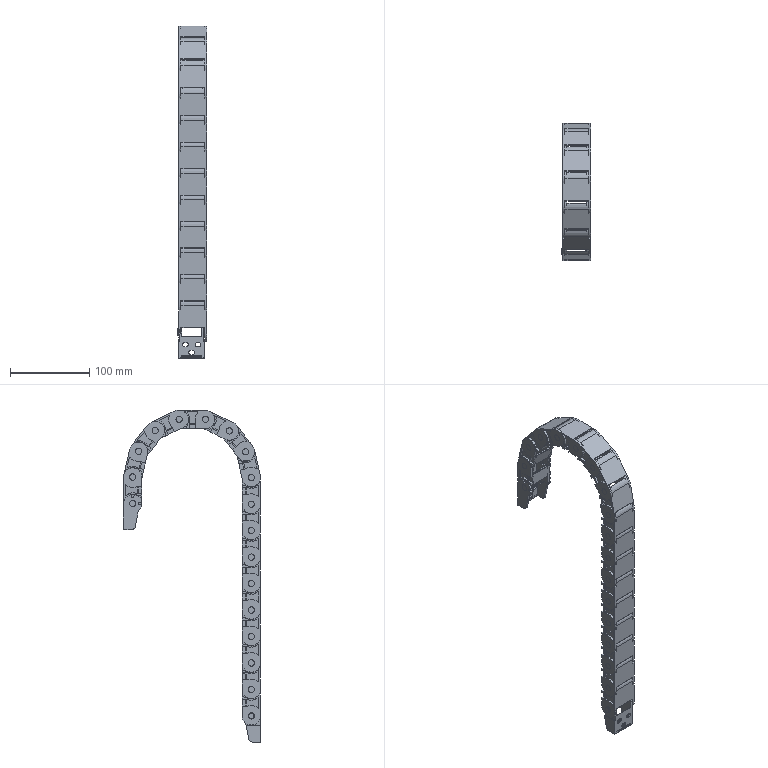Part | 19 solids | 2565 faces | box 37.15 x 173.38 x 420.141 mm | volume 170275 mm3 | plane 1457 | cylinder 1092 | cone 12 | torus 4 | commonest cylinder face diameters 2 x204 1 x170 0.6 x136 23.26 x119 11.94 x102 24.06 x85